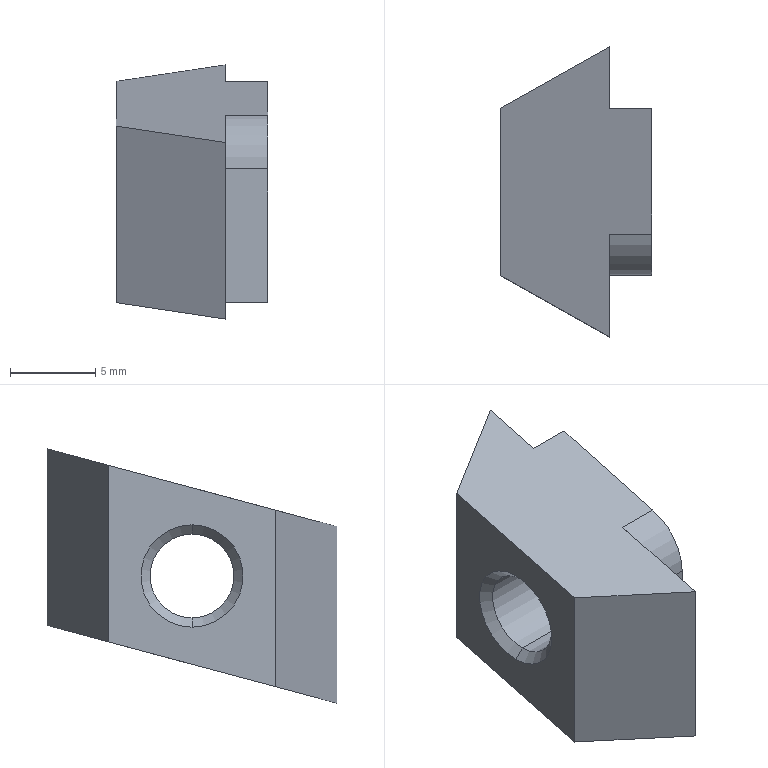Part | STEP file | 0245_019_HNTFSN8-6 | 1 solid | 18 faces | box 8.9 x 17 x 14.908 mm | volume 961.616 mm3 | plane 10 | cone 4 | cylinder 4 | commonest cylinder face diameters 4.917 x2 6.533 x2
STEP:
#1=CARTESIAN_POINT('',(0.,0.,0.));
#2=DIRECTION('',(0.,0.,1.));
#3=DIRECTION('',(1.,0.,0.));
#4=AXIS2_PLACEMENT_3D('',#1,#2,#3);
#5=CARTESIAN_POINT('',(-8.358,0.,2.459));
#6=VERTEX_POINT('',#5);
#7=CARTESIAN_POINT('',(-8.9,0.,3.));
#8=VERTEX_POINT('',#7);
#9=CARTESIAN_POINT('',(-8.9,0.,3.));
#10=DIRECTION('',(-0.7071,0.,0.7071));
#11=VECTOR('',#10,1.);
#12=LINE('',#9,#11);
#13=CARTESIAN_POINT('',(-8.9,0.,0.));
#14=DIRECTION('',(-1.,0.,0.));
#15=DIRECTION('',(0.,0.,1.));
#16=AXIS2_PLACEMENT_3D('',#13,#14,#15);
#17=CONICAL_SURFACE('',#16,3.,0.7854);
#18=CARTESIAN_POINT('',(6.283,0.));
#19=DIRECTION('',(0.,1.));
#20=VECTOR('',#19,1.);
#21=LINE('',#18,#20);
#22=(GEOMETRIC_REPRESENTATION_CONTEXT(2)PARAMETRIC_REPRESENTATION_CONTEXT()REPRESENTATION_CONTEXT('',''));
#23=DEFINITIONAL_REPRESENTATION('',(#21),#22);
#24=PCURVE('',#17,#23);
#25=CARTESIAN_POINT('',(-8.9,0.,0.));
#26=DIRECTION('',(-1.,0.,0.));
#27=DIRECTION('',(0.,0.,1.));
#28=AXIS2_PLACEMENT_3D('',#25,#26,#27);
#29=CONICAL_SURFACE('',#28,3.,0.7854);
#30=CARTESIAN_POINT('',(0.,0.));
#31=DIRECTION('',(0.,1.));
#32=VECTOR('',#31,1.);
#33=LINE('',#30,#32);
#34=(GEOMETRIC_REPRESENTATION_CONTEXT(2)PARAMETRIC_REPRESENTATION_CONTEXT()REPRESENTATION_CONTEXT('',''));
#35=DEFINITIONAL_REPRESENTATION('',(#33),#34);
#36=PCURVE('',#29,#35);
#37=SURFACE_CURVE('',#12,(#24,#36),.PCURVE_S1.);
#38=EDGE_CURVE('',#6,#8,#37,.T.);
#39=ORIENTED_EDGE('',*,*,#38,.T.);
#40=CARTESIAN_POINT('',(-8.9,0.,-3.));
#41=VERTEX_POINT('',#40);
#42=CARTESIAN_POINT('',(-8.9,0.,0.));
#43=DIRECTION('',(-1.,0.,0.));
#44=DIRECTION('',(0.,0.,1.));
#45=AXIS2_PLACEMENT_3D('',#42,#43,#44);
#46=CIRCLE('',#45,3.);
#47=CARTESIAN_POINT('',(0.,0.));
#48=DIRECTION('',(1.,0.));
#49=VECTOR('',#48,1.);
#50=LINE('',#47,#49);
#51=(GEOMETRIC_REPRESENTATION_CONTEXT(2)PARAMETRIC_REPRESENTATION_CONTEXT()REPRESENTATION_CONTEXT('',''));
#52=DEFINITIONAL_REPRESENTATION('',(#50),#51);
#53=PCURVE('',#17,#52);
#54=CARTESIAN_POINT('',(-8.9,0.,0.));
#55=DIRECTION('',(1.,0.,0.));
#56=DIRECTION('',(0.,0.,-1.));
#57=AXIS2_PLACEMENT_3D('',#54,#55,#56);
#58=PLANE('',#57);
#59=CARTESIAN_POINT('',(-3.,0.));
#60=CARTESIAN_POINT('',(-3.,5.196));
#61=CARTESIAN_POINT('',(1.5,2.598));
#62=CARTESIAN_POINT('',(6.,0.));
#63=CARTESIAN_POINT('',(1.5,-2.598));
#64=CARTESIAN_POINT('',(-3.,-5.196));
#65=CARTESIAN_POINT('',(-3.,0.));
#66=(BOUNDED_CURVE()B_SPLINE_CURVE(2,(#59,#60,#61,#62,#63,#64,#65),.UNSPECIFIED.,.T.,.F.)B_SPLINE_CURVE_WITH_KNOTS((1,2,2,2,2,1),(-2.094,0.,2.094,4.189,6.283,8.378),.UNSPECIFIED.)CURVE()GEOMETRIC_REPRESENTATION_ITEM()RATIONAL_B_SPLINE_CURVE((1.,0.5,1.,0.5,1.,0.5,1.))REPRESENTATION_ITEM(''));
#67=(GEOMETRIC_REPRESENTATION_CONTEXT(2)PARAMETRIC_REPRESENTATION_CONTEXT()REPRESENTATION_CONTEXT('',''));
#68=DEFINITIONAL_REPRESENTATION('',(#66),#67);
#69=PCURVE('',#58,#68);
#70=SURFACE_CURVE('',#46,(#53,#69),.PCURVE_S1.);
#71=EDGE_CURVE('',#41,#8,#70,.T.);
#72=ORIENTED_EDGE('',*,*,#71,.F.);
#73=CARTESIAN_POINT('',(-8.358,0.,-2.459));
#74=VERTEX_POINT('',#73);
#75=CARTESIAN_POINT('',(-8.9,0.,-3.));
#76=DIRECTION('',(-0.7071,0.,-0.7071));
#77=VECTOR('',#76,1.);
#78=LINE('',#75,#77);
#79=CARTESIAN_POINT('',(3.142,0.));
#80=DIRECTION('',(0.,1.));
#81=VECTOR('',#80,1.);
#82=LINE('',#79,#81);
#83=(GEOMETRIC_REPRESENTATION_CONTEXT(2)PARAMETRIC_REPRESENTATION_CONTEXT()REPRESENTATION_CONTEXT('',''));
#84=DEFINITIONAL_REPRESENTATION('',(#82),#83);
#85=PCURVE('',#17,#84);
#86=CARTESIAN_POINT('',(3.142,0.));
#87=DIRECTION('',(0.,1.));
#88=VECTOR('',#87,1.);
#89=LINE('',#86,#88);
#90=(GEOMETRIC_REPRESENTATION_CONTEXT(2)PARAMETRIC_REPRESENTATION_CONTEXT()REPRESENTATION_CONTEXT('',''));
#91=DEFINITIONAL_REPRESENTATION('',(#89),#90);
#92=PCURVE('',#29,#91);
#93=SURFACE_CURVE('',#78,(#85,#92),.PCURVE_S1.);
#94=EDGE_CURVE('',#74,#41,#93,.T.);
#95=ORIENTED_EDGE('',*,*,#94,.F.);
#96=CARTESIAN_POINT('',(-8.358,0.,0.));
#97=DIRECTION('',(-1.,0.,0.));
#98=DIRECTION('',(0.,1.,0.));
#99=AXIS2_PLACEMENT_3D('',#96,#97,#98);
#100=CIRCLE('',#99,2.459);
#101=CARTESIAN_POINT('',(1.571,-0.5415));
#102=DIRECTION('',(1.,0.));
#103=VECTOR('',#102,1.);
#104=LINE('',#101,#103);
#105=(GEOMETRIC_REPRESENTATION_CONTEXT(2)PARAMETRIC_REPRESENTATION_CONTEXT()REPRESENTATION_CONTEXT('',''));
#106=DEFINITIONAL_REPRESENTATION('',(#104),#105);
#107=PCURVE('',#17,#106);
#108=CARTESIAN_POINT('',(-4.45,0.,0.));
#109=DIRECTION('',(1.,0.,0.));
#110=DIRECTION('',(0.,0.,-1.));
#111=AXIS2_PLACEMENT_3D('',#108,#109,#110);
#112=CYLINDRICAL_SURFACE('',#111,2.458);
#113=CARTESIAN_POINT('',(7.854,-3.908));
#114=DIRECTION('',(-1.,0.));
#115=VECTOR('',#114,1.);
#116=LINE('',#113,#115);
#117=(GEOMETRIC_REPRESENTATION_CONTEXT(2)PARAMETRIC_REPRESENTATION_CONTEXT()REPRESENTATION_CONTEXT('',''));
#118=DEFINITIONAL_REPRESENTATION('',(#116),#117);
#119=PCURVE('',#112,#118);
#120=SURFACE_CURVE('',#100,(#107,#119),.PCURVE_S1.);
#121=EDGE_CURVE('',#74,#6,#120,.T.);
#122=ORIENTED_EDGE('',*,*,#121,.T.);
#123=EDGE_LOOP('',(#39,#72,#95,#122));
#124=FACE_BOUND('',#123,.F.);
#125=ADVANCED_FACE('',(#124),#17,.F.);
#126=CARTESIAN_POINT('',(-0.5415,0.,-2.458));
#127=VERTEX_POINT('',#126);
#128=CARTESIAN_POINT('',(0.,0.,-3.));
#129=VERTEX_POINT('',#128);
#130=CARTESIAN_POINT('',(0.,0.,-3.));
#131=DIRECTION('',(0.7071,0.,-0.7071));
#132=VECTOR('',#131,1.);
#133=LINE('',#130,#132);
#134=CARTESIAN_POINT('',(0.,0.,0.));
#135=DIRECTION('',(1.,0.,0.));
#136=DIRECTION('',(0.,0.,-1.));
#137=AXIS2_PLACEMENT_3D('',#134,#135,#136);
#138=CONICAL_SURFACE('',#137,3.,0.7854);
#139=CARTESIAN_POINT('',(6.283,0.));
#140=DIRECTION('',(0.,1.));
#141=VECTOR('',#140,1.);
#142=LINE('',#139,#141);
#143=(GEOMETRIC_REPRESENTATION_CONTEXT(2)PARAMETRIC_REPRESENTATION_CONTEXT()REPRESENTATION_CONTEXT('',''));
#144=DEFINITIONAL_REPRESENTATION('',(#142),#143);
#145=PCURVE('',#138,#144);
#146=CARTESIAN_POINT('',(0.,0.,0.));
#147=DIRECTION('',(1.,0.,0.));
#148=DIRECTION('',(0.,0.,-1.));
#149=AXIS2_PLACEMENT_3D('',#146,#147,#148);
#150=CONICAL_SURFACE('',#149,3.,0.7854);
#151=CARTESIAN_POINT('',(0.,0.));
#152=DIRECTION('',(0.,1.));
#153=VECTOR('',#152,1.);
#154=LINE('',#151,#153);
#155=(GEOMETRIC_REPRESENTATION_CONTEXT(2)PARAMETRIC_REPRESENTATION_CONTEXT()REPRESENTATION_CONTEXT('',''));
#156=DEFINITIONAL_REPRESENTATION('',(#154),#155);
#157=PCURVE('',#150,#156);
#158=SURFACE_CURVE('',#133,(#145,#157),.PCURVE_S1.);
#159=EDGE_CURVE('',#127,#129,#158,.T.);
#160=ORIENTED_EDGE('',*,*,#159,.T.);
#161=CARTESIAN_POINT('',(0.,0.,3.));
#162=VERTEX_POINT('',#161);
#163=CARTESIAN_POINT('',(0.,0.,0.));
#164=DIRECTION('',(-1.,0.,0.));
#165=DIRECTION('',(0.,0.,-1.));
#166=AXIS2_PLACEMENT_3D('',#163,#164,#165);
#167=CIRCLE('',#166,3.);
#168=CARTESIAN_POINT('',(6.283,0.));
#169=DIRECTION('',(-1.,0.));
#170=VECTOR('',#169,1.);
#171=LINE('',#168,#170);
#172=(GEOMETRIC_REPRESENTATION_CONTEXT(2)PARAMETRIC_REPRESENTATION_CONTEXT()REPRESENTATION_CONTEXT('',''));
#173=DEFINITIONAL_REPRESENTATION('',(#171),#172);
#174=PCURVE('',#138,#173);
#175=CARTESIAN_POINT('',(0.,0.,0.));
#176=DIRECTION('',(1.,0.,0.));
#177=DIRECTION('',(0.,0.,-1.));
#178=AXIS2_PLACEMENT_3D('',#175,#176,#177);
#179=PLANE('',#178);
#180=CARTESIAN_POINT('',(3.,0.));
#181=CARTESIAN_POINT('',(3.,-5.196));
#182=CARTESIAN_POINT('',(-1.5,-2.598));
#183=CARTESIAN_POINT('',(-6.,0.));
#184=CARTESIAN_POINT('',(-1.5,2.598));
#185=CARTESIAN_POINT('',(3.,5.196));
#186=CARTESIAN_POINT('',(3.,0.));
#187=(BOUNDED_CURVE()B_SPLINE_CURVE(2,(#180,#181,#182,#183,#184,#185,#186),.UNSPECIFIED.,.T.,.F.)B_SPLINE_CURVE_WITH_KNOTS((1,2,2,2,2,1),(-2.094,0.,2.094,4.189,6.283,8.378),.UNSPECIFIED.)CURVE()GEOMETRIC_REPRESENTATION_ITEM()RATIONAL_B_SPLINE_CURVE((1.,0.5,1.,0.5,1.,0.5,1.))REPRESENTATION_ITEM(''));
#188=(GEOMETRIC_REPRESENTATION_CONTEXT(2)PARAMETRIC_REPRESENTATION_CONTEXT()REPRESENTATION_CONTEXT('',''));
#189=DEFINITIONAL_REPRESENTATION('',(#187),#188);
#190=PCURVE('',#179,#189);
#191=SURFACE_CURVE('',#167,(#174,#190),.PCURVE_S1.);
#192=EDGE_CURVE('',#129,#162,#191,.T.);
#193=ORIENTED_EDGE('',*,*,#192,.T.);
#194=CARTESIAN_POINT('',(-0.5415,0.,2.458));
#195=VERTEX_POINT('',#194);
#196=CARTESIAN_POINT('',(0.,0.,3.));
#197=DIRECTION('',(0.7071,0.,0.7071));
#198=VECTOR('',#197,1.);
#199=LINE('',#196,#198);
#200=CARTESIAN_POINT('',(3.142,0.));
#201=DIRECTION('',(0.,1.));
#202=VECTOR('',#201,1.);
#203=LINE('',#200,#202);
#204=(GEOMETRIC_REPRESENTATION_CONTEXT(2)PARAMETRIC_REPRESENTATION_CONTEXT()REPRESENTATION_CONTEXT('',''));
#205=DEFINITIONAL_REPRESENTATION('',(#203),#204);
#206=PCURVE('',#138,#205);
#207=CARTESIAN_POINT('',(3.142,0.));
#208=DIRECTION('',(0.,1.));
#209=VECTOR('',#208,1.);
#210=LINE('',#207,#209);
#211=(GEOMETRIC_REPRESENTATION_CONTEXT(2)PARAMETRIC_REPRESENTATION_CONTEXT()REPRESENTATION_CONTEXT('',''));
#212=DEFINITIONAL_REPRESENTATION('',(#210),#211);
#213=PCURVE('',#150,#212);
#214=SURFACE_CURVE('',#199,(#206,#213),.PCURVE_S1.);
#215=EDGE_CURVE('',#195,#162,#214,.T.);
#216=ORIENTED_EDGE('',*,*,#215,.F.);
#217=CARTESIAN_POINT('',(-0.5415,0.,0.));
#218=DIRECTION('',(1.,0.,0.));
#219=DIRECTION('',(0.,1.,0.));
#220=AXIS2_PLACEMENT_3D('',#217,#218,#219);
#221=CIRCLE('',#220,2.458);
#222=CARTESIAN_POINT('',(1.571,-0.5415));
#223=DIRECTION('',(1.,0.));
#224=VECTOR('',#223,1.);
#225=LINE('',#222,#224);
#226=(GEOMETRIC_REPRESENTATION_CONTEXT(2)PARAMETRIC_REPRESENTATION_CONTEXT()REPRESENTATION_CONTEXT('',''));
#227=DEFINITIONAL_REPRESENTATION('',(#225),#226);
#228=PCURVE('',#138,#227);
#229=CARTESIAN_POINT('',(1.571,3.908));
#230=DIRECTION('',(1.,0.));
#231=VECTOR('',#230,1.);
#232=LINE('',#229,#231);
#233=(GEOMETRIC_REPRESENTATION_CONTEXT(2)PARAMETRIC_REPRESENTATION_CONTEXT()REPRESENTATION_CONTEXT('',''));
#234=DEFINITIONAL_REPRESENTATION('',(#232),#233);
#235=PCURVE('',#112,#234);
#236=SURFACE_CURVE('',#221,(#228,#235),.PCURVE_S1.);
#237=EDGE_CURVE('',#195,#127,#236,.T.);
#238=ORIENTED_EDGE('',*,*,#237,.T.);
#239=EDGE_LOOP('',(#160,#193,#216,#238));
#240=FACE_BOUND('',#239,.F.);
#241=ADVANCED_FACE('',(#240),#138,.F.);
#242=CARTESIAN_POINT('',(-4.45,0.,-2.458));
#243=DIRECTION('',(1.,0.,0.));
#244=VECTOR('',#243,1.);
#245=LINE('',#242,#244);
#246=CARTESIAN_POINT('',(6.283,0.));
#247=DIRECTION('',(0.,1.));
#248=VECTOR('',#247,1.);
#249=LINE('',#246,#248);
#250=(GEOMETRIC_REPRESENTATION_CONTEXT(2)PARAMETRIC_REPRESENTATION_CONTEXT()REPRESENTATION_CONTEXT('',''));
#251=DEFINITIONAL_REPRESENTATION('',(#249),#250);
#252=PCURVE('',#112,#251);
#253=CARTESIAN_POINT('',(-4.45,0.,0.));
#254=DIRECTION('',(1.,0.,0.));
#255=DIRECTION('',(0.,0.,-1.));
#256=AXIS2_PLACEMENT_3D('',#253,#254,#255);
#257=CYLINDRICAL_SURFACE('',#256,2.458);
#258=CARTESIAN_POINT('',(0.,0.));
#259=DIRECTION('',(0.,1.));
#260=VECTOR('',#259,1.);
#261=LINE('',#258,#260);
#262=(GEOMETRIC_REPRESENTATION_CONTEXT(2)PARAMETRIC_REPRESENTATION_CONTEXT()REPRESENTATION_CONTEXT('',''));
#263=DEFINITIONAL_REPRESENTATION('',(#261),#262);
#264=PCURVE('',#257,#263);
#265=SURFACE_CURVE('',#245,(#252,#264),.PCURVE_S1.);
#266=EDGE_CURVE('',#74,#127,#265,.T.);
#267=ORIENTED_EDGE('',*,*,#266,.T.);
#268=ORIENTED_EDGE('',*,*,#237,.F.);
#269=CARTESIAN_POINT('',(-4.45,0.,2.458));
#270=DIRECTION('',(1.,0.,0.));
#271=VECTOR('',#270,1.);
#272=LINE('',#269,#271);
#273=CARTESIAN_POINT('',(3.142,0.));
#274=DIRECTION('',(0.,1.));
#275=VECTOR('',#274,1.);
#276=LINE('',#273,#275);
#277=(GEOMETRIC_REPRESENTATION_CONTEXT(2)PARAMETRIC_REPRESENTATION_CONTEXT()REPRESENTATION_CONTEXT('',''));
#278=DEFINITIONAL_REPRESENTATION('',(#276),#277);
#279=PCURVE('',#112,#278);
#280=CARTESIAN_POINT('',(3.142,0.));
#281=DIRECTION('',(0.,1.));
#282=VECTOR('',#281,1.);
#283=LINE('',#280,#282);
#284=(GEOMETRIC_REPRESENTATION_CONTEXT(2)PARAMETRIC_REPRESENTATION_CONTEXT()REPRESENTATION_CONTEXT('',''));
#285=DEFINITIONAL_REPRESENTATION('',(#283),#284);
#286=PCURVE('',#257,#285);
#287=SURFACE_CURVE('',#272,(#279,#286),.PCURVE_S1.);
#288=EDGE_CURVE('',#6,#195,#287,.T.);
#289=ORIENTED_EDGE('',*,*,#288,.F.);
#290=ORIENTED_EDGE('',*,*,#121,.F.);
#291=EDGE_LOOP('',(#267,#268,#289,#290));
#292=FACE_BOUND('',#291,.F.);
#293=ADVANCED_FACE('',(#292),#112,.F.);
#294=CARTESIAN_POINT('',(-8.9,-4.9,3.863));
#295=VERTEX_POINT('',#294);
#296=CARTESIAN_POINT('',(-2.5,-8.5,2.899));
#297=VERTEX_POINT('',#296);
#298=CARTESIAN_POINT('',(-8.9,-4.9,3.863));
#299=DIRECTION('',(0.8642,-0.4861,-0.1302));
#300=VECTOR('',#299,1.);
#301=LINE('',#298,#300);
#302=CARTESIAN_POINT('',(0.,8.5,7.454));
#303=DIRECTION('',(0.,-0.2588,0.9659));
#304=DIRECTION('',(0.,-0.9659,-0.2588));
#305=AXIS2_PLACEMENT_3D('',#302,#303,#304);
#306=PLANE('',#305);
#307=CARTESIAN_POINT('',(13.873,-8.9));
#308=DIRECTION('',(0.5032,0.8642));
#309=VECTOR('',#308,1.);
#310=LINE('',#307,#309);
#311=(GEOMETRIC_REPRESENTATION_CONTEXT(2)PARAMETRIC_REPRESENTATION_CONTEXT()REPRESENTATION_CONTEXT('',''));
#312=DEFINITIONAL_REPRESENTATION('',(#310),#311);
#313=PCURVE('',#306,#312);
#314=CARTESIAN_POINT('',(-2.5,-8.5,20.));
#315=DIRECTION('',(0.4903,0.8716,0.));
#316=DIRECTION('',(-0.8716,0.4903,0.));
#317=AXIS2_PLACEMENT_3D('',#314,#315,#316);
#318=PLANE('',#317);
#319=CARTESIAN_POINT('',(7.343,-16.137));
#320=DIRECTION('',(-0.9915,-0.1302));
#321=VECTOR('',#320,1.);
#322=LINE('',#319,#321);
#323=(GEOMETRIC_REPRESENTATION_CONTEXT(2)PARAMETRIC_REPRESENTATION_CONTEXT()REPRESENTATION_CONTEXT('',''));
#324=DEFINITIONAL_REPRESENTATION('',(#322),#323);
#325=PCURVE('',#318,#324);
#326=SURFACE_CURVE('',#301,(#313,#325),.PCURVE_S1.);
#327=EDGE_CURVE('',#295,#297,#326,.T.);
#328=ORIENTED_EDGE('',*,*,#327,.T.);
#329=CARTESIAN_POINT('',(-2.5,-2.479,4.512));
#330=VERTEX_POINT('',#329);
#331=CARTESIAN_POINT('',(-2.5,8.5,7.454));
#332=DIRECTION('',(0.,0.9659,0.2588));
#333=VECTOR('',#332,1.);
#334=LINE('',#331,#333);
#335=CARTESIAN_POINT('',(0.,-2.5));
#336=DIRECTION('',(-1.,0.));
#337=VECTOR('',#336,1.);
#338=LINE('',#335,#337);
#339=(GEOMETRIC_REPRESENTATION_CONTEXT(2)PARAMETRIC_REPRESENTATION_CONTEXT()REPRESENTATION_CONTEXT('',''));
#340=DEFINITIONAL_REPRESENTATION('',(#338),#339);
#341=PCURVE('',#306,#340);
#342=CARTESIAN_POINT('',(-2.5,-4.9,20.));
#343=DIRECTION('',(-1.,0.,0.));
#344=DIRECTION('',(0.,0.,1.));
#345=AXIS2_PLACEMENT_3D('',#342,#343,#344);
#346=PLANE('',#345);
#347=CARTESIAN_POINT('',(-12.546,13.4));
#348=DIRECTION('',(0.2588,0.9659));
#349=VECTOR('',#348,1.);
#350=LINE('',#347,#349);
#351=(GEOMETRIC_REPRESENTATION_CONTEXT(2)PARAMETRIC_REPRESENTATION_CONTEXT()REPRESENTATION_CONTEXT('',''));
#352=DEFINITIONAL_REPRESENTATION('',(#350),#351);
#353=PCURVE('',#346,#352);
#354=SURFACE_CURVE('',#334,(#341,#353),.PCURVE_S1.);
#355=EDGE_CURVE('',#297,#330,#354,.T.);
#356=ORIENTED_EDGE('',*,*,#355,.T.);
#357=CARTESIAN_POINT('',(0.,-2.479,4.512));
#358=VERTEX_POINT('',#357);
#359=CARTESIAN_POINT('',(0.,-2.479,4.512));
#360=DIRECTION('',(1.,0.,0.));
#361=VECTOR('',#360,1.);
#362=LINE('',#359,#361);
#363=CARTESIAN_POINT('',(11.366,0.));
#364=DIRECTION('',(0.,1.));
#365=VECTOR('',#364,1.);
#366=LINE('',#363,#365);
#367=(GEOMETRIC_REPRESENTATION_CONTEXT(2)PARAMETRIC_REPRESENTATION_CONTEXT()REPRESENTATION_CONTEXT('',''));
#368=DEFINITIONAL_REPRESENTATION('',(#366),#367);
#369=PCURVE('',#306,#368);
#370=CARTESIAN_POINT('',(-2.5,-1.633,1.357));
#371=DIRECTION('',(-1.,0.,0.));
#372=DIRECTION('',(0.,0.,1.));
#373=AXIS2_PLACEMENT_3D('',#370,#371,#372);
#374=CYLINDRICAL_SURFACE('',#373,3.267);
#375=CARTESIAN_POINT('',(6.021,-2.5));
#376=DIRECTION('',(0.,-1.));
#377=VECTOR('',#376,1.);
#378=LINE('',#375,#377);
#379=(GEOMETRIC_REPRESENTATION_CONTEXT(2)PARAMETRIC_REPRESENTATION_CONTEXT()REPRESENTATION_CONTEXT('',''));
#380=DEFINITIONAL_REPRESENTATION('',(#378),#379);
#381=PCURVE('',#374,#380);
#382=SURFACE_CURVE('',#362,(#369,#381),.PCURVE_S1.);
#383=EDGE_CURVE('',#330,#358,#382,.T.);
#384=ORIENTED_EDGE('',*,*,#383,.T.);
#385=CARTESIAN_POINT('',(0.,4.9,6.489));
#386=VERTEX_POINT('',#385);
#387=CARTESIAN_POINT('',(0.,8.5,7.454));
#388=DIRECTION('',(0.,0.9659,0.2588));
#389=VECTOR('',#388,1.);
#390=LINE('',#387,#389);
#391=CARTESIAN_POINT('',(0.,0.));
#392=DIRECTION('',(-1.,0.));
#393=VECTOR('',#392,1.);
#394=LINE('',#391,#393);
#395=(GEOMETRIC_REPRESENTATION_CONTEXT(2)PARAMETRIC_REPRESENTATION_CONTEXT()REPRESENTATION_CONTEXT('',''));
#396=DEFINITIONAL_REPRESENTATION('',(#394),#395);
#397=PCURVE('',#306,#396);
#398=CARTESIAN_POINT('',(-7.454,8.5));
#399=DIRECTION('',(-0.2588,0.9659));
#400=VECTOR('',#399,1.);
#401=LINE('',#398,#400);
#402=(GEOMETRIC_REPRESENTATION_CONTEXT(2)PARAMETRIC_REPRESENTATION_CONTEXT()REPRESENTATION_CONTEXT('',''));
#403=DEFINITIONAL_REPRESENTATION('',(#401),#402);
#404=PCURVE('',#179,#403);
#405=SURFACE_CURVE('',#390,(#397,#404),.PCURVE_S1.);
#406=EDGE_CURVE('',#358,#386,#405,.T.);
#407=ORIENTED_EDGE('',*,*,#406,.T.);
#408=CARTESIAN_POINT('',(-2.5,4.9,6.489));
#409=VERTEX_POINT('',#408);
#410=CARTESIAN_POINT('',(0.,4.9,6.489));
#411=DIRECTION('',(-1.,0.,0.));
#412=VECTOR('',#411,1.);
#413=LINE('',#410,#412);
#414=CARTESIAN_POINT('',(3.727,0.));
#415=DIRECTION('',(0.,-1.));
#416=VECTOR('',#415,1.);
#417=LINE('',#414,#416);
#418=(GEOMETRIC_REPRESENTATION_CONTEXT(2)PARAMETRIC_REPRESENTATION_CONTEXT()REPRESENTATION_CONTEXT('',''));
#419=DEFINITIONAL_REPRESENTATION('',(#417),#418);
#420=PCURVE('',#306,#419);
#421=CARTESIAN_POINT('',(-2.5,4.9,20.));
#422=DIRECTION('',(0.,-1.,0.));
#423=DIRECTION('',(1.,0.,0.));
#424=AXIS2_PLACEMENT_3D('',#421,#422,#423);
#425=PLANE('',#424);
#426=CARTESIAN_POINT('',(2.5,-13.511));
#427=DIRECTION('',(-1.,0.));
#428=VECTOR('',#427,1.);
#429=LINE('',#426,#428);
#430=(GEOMETRIC_REPRESENTATION_CONTEXT(2)PARAMETRIC_REPRESENTATION_CONTEXT()REPRESENTATION_CONTEXT('',''));
#431=DEFINITIONAL_REPRESENTATION('',(#429),#430);
#432=PCURVE('',#425,#431);
#433=SURFACE_CURVE('',#413,(#420,#432),.PCURVE_S1.);
#434=EDGE_CURVE('',#386,#409,#433,.T.);
#435=ORIENTED_EDGE('',*,*,#434,.T.);
#436=CARTESIAN_POINT('',(-2.5,8.5,7.454));
#437=VERTEX_POINT('',#436);
#438=CARTESIAN_POINT('',(-2.5,8.5,7.454));
#439=DIRECTION('',(0.,0.9659,0.2588));
#440=VECTOR('',#439,1.);
#441=LINE('',#438,#440);
#442=CARTESIAN_POINT('',(0.,-2.5));
#443=DIRECTION('',(-1.,0.));
#444=VECTOR('',#443,1.);
#445=LINE('',#442,#444);
#446=(GEOMETRIC_REPRESENTATION_CONTEXT(2)PARAMETRIC_REPRESENTATION_CONTEXT()REPRESENTATION_CONTEXT('',''));
#447=DEFINITIONAL_REPRESENTATION('',(#445),#446);
#448=PCURVE('',#306,#447);
#449=CARTESIAN_POINT('',(-2.5,8.5,20.));
#450=DIRECTION('',(-1.,0.,0.));
#451=DIRECTION('',(0.,0.,1.));
#452=AXIS2_PLACEMENT_3D('',#449,#450,#451);
#453=PLANE('',#452);
#454=CARTESIAN_POINT('',(-12.546,0.));
#455=DIRECTION('',(0.2588,0.9659));
#456=VECTOR('',#455,1.);
#457=LINE('',#454,#456);
#458=(GEOMETRIC_REPRESENTATION_CONTEXT(2)PARAMETRIC_REPRESENTATION_CONTEXT()REPRESENTATION_CONTEXT('',''));
#459=DEFINITIONAL_REPRESENTATION('',(#457),#458);
#460=PCURVE('',#453,#459);
#461=SURFACE_CURVE('',#441,(#448,#460),.PCURVE_S1.);
#462=EDGE_CURVE('',#409,#437,#461,.T.);
#463=ORIENTED_EDGE('',*,*,#462,.T.);
#464=CARTESIAN_POINT('',(-8.9,4.9,6.489));
#465=VERTEX_POINT('',#464);
#466=CARTESIAN_POINT('',(-2.5,8.5,7.454));
#467=DIRECTION('',(-0.8642,-0.4861,-0.1302));
#468=VECTOR('',#467,1.);
#469=LINE('',#466,#468);
#470=CARTESIAN_POINT('',(0.,-2.5));
#471=DIRECTION('',(0.5032,-0.8642));
#472=VECTOR('',#471,1.);
#473=LINE('',#470,#472);
#474=(GEOMETRIC_REPRESENTATION_CONTEXT(2)PARAMETRIC_REPRESENTATION_CONTEXT()REPRESENTATION_CONTEXT('',''));
#475=DEFINITIONAL_REPRESENTATION('',(#473),#474);
#476=PCURVE('',#306,#475);
#477=CARTESIAN_POINT('',(-8.9,4.9,20.));
#478=DIRECTION('',(0.4903,-0.8716,0.));
#479=DIRECTION('',(0.8716,0.4903,0.));
#480=AXIS2_PLACEMENT_3D('',#477,#478,#479);
#481=PLANE('',#480);
#482=CARTESIAN_POINT('',(7.343,-12.546));
#483=DIRECTION('',(-0.9915,-0.1302));
#484=VECTOR('',#483,1.);
#485=LINE('',#482,#484);
#486=(GEOMETRIC_REPRESENTATION_CONTEXT(2)PARAMETRIC_REPRESENTATION_CONTEXT()REPRESENTATION_CONTEXT('',''));
#487=DEFINITIONAL_REPRESENTATION('',(#485),#486);
#488=PCURVE('',#481,#487);
#489=SURFACE_CURVE('',#469,(#476,#488),.PCURVE_S1.);
#490=EDGE_CURVE('',#437,#465,#489,.T.);
#491=ORIENTED_EDGE('',*,*,#490,.T.);
#492=CARTESIAN_POINT('',(-8.9,8.5,7.454));
#493=DIRECTION('',(0.,-0.9659,-0.2588));
#494=VECTOR('',#493,1.);
#495=LINE('',#492,#494);
#496=CARTESIAN_POINT('',(0.,-8.9));
#497=DIRECTION('',(1.,0.));
#498=VECTOR('',#497,1.);
#499=LINE('',#496,#498);
#500=(GEOMETRIC_REPRESENTATION_CONTEXT(2)PARAMETRIC_REPRESENTATION_CONTEXT()REPRESENTATION_CONTEXT('',''));
#501=DEFINITIONAL_REPRESENTATION('',(#499),#500);
#502=PCURVE('',#306,#501);
#503=CARTESIAN_POINT('',(-7.454,8.5));
#504=DIRECTION('',(0.2588,-0.9659));
#505=VECTOR('',#504,1.);
#506=LINE('',#503,#505);
#507=(GEOMETRIC_REPRESENTATION_CONTEXT(2)PARAMETRIC_REPRESENTATION_CONTEXT()REPRESENTATION_CONTEXT('',''));
#508=DEFINITIONAL_REPRESENTATION('',(#506),#507);
#509=PCURVE('',#58,#508);
#510=SURFACE_CURVE('',#495,(#502,#509),.PCURVE_S1.);
#511=EDGE_CURVE('',#465,#295,#510,.T.);
#512=ORIENTED_EDGE('',*,*,#511,.T.);
#513=EDGE_LOOP('',(#328,#356,#384,#407,#435,#463,#491,#512));
#514=FACE_BOUND('',#513,.T.);
#515=ADVANCED_FACE('',(#514),#306,.T.);
#516=CARTESIAN_POINT('',(-2.5,-8.5,-7.454));
#517=VERTEX_POINT('',#516);
#518=CARTESIAN_POINT('',(-2.5,-8.5,20.));
#519=DIRECTION('',(0.,0.,1.));
#520=VECTOR('',#519,1.);
#521=LINE('',#518,#520);
#522=CARTESIAN_POINT('',(0.,-3.6));
#523=DIRECTION('',(1.,0.));
#524=VECTOR('',#523,1.);
#525=LINE('',#522,#524);
#526=(GEOMETRIC_REPRESENTATION_CONTEXT(2)PARAMETRIC_REPRESENTATION_CONTEXT()REPRESENTATION_CONTEXT('',''));
#527=DEFINITIONAL_REPRESENTATION('',(#525),#526);
#528=PCURVE('',#346,#527);
#529=CARTESIAN_POINT('',(0.,0.));
#530=DIRECTION('',(0.,1.));
#531=VECTOR('',#530,1.);
#532=LINE('',#529,#531);
#533=(GEOMETRIC_REPRESENTATION_CONTEXT(2)PARAMETRIC_REPRESENTATION_CONTEXT()REPRESENTATION_CONTEXT('',''));
#534=DEFINITIONAL_REPRESENTATION('',(#532),#533);
#535=PCURVE('',#318,#534);
#536=SURFACE_CURVE('',#521,(#528,#535),.PCURVE_S1.);
#537=EDGE_CURVE('',#517,#297,#536,.T.);
#538=ORIENTED_EDGE('',*,*,#537,.F.);
#539=CARTESIAN_POINT('',(-2.5,-4.9,-6.489));
#540=VERTEX_POINT('',#539);
#541=CARTESIAN_POINT('',(-2.5,-4.9,-6.489));
#542=DIRECTION('',(0.,-0.9659,-0.2588));
#543=VECTOR('',#542,1.);
#544=LINE('',#541,#543);
#545=CARTESIAN_POINT('',(-26.489,0.));
#546=DIRECTION('',(-0.2588,-0.9659));
#547=VECTOR('',#546,1.);
#548=LINE('',#545,#547);
#549=(GEOMETRIC_REPRESENTATION_CONTEXT(2)PARAMETRIC_REPRESENTATION_CONTEXT()REPRESENTATION_CONTEXT('',''));
#550=DEFINITIONAL_REPRESENTATION('',(#548),#549);
#551=PCURVE('',#346,#550);
#552=CARTESIAN_POINT('',(0.,-8.5,-7.454));
#553=DIRECTION('',(0.,0.2588,-0.9659));
#554=DIRECTION('',(0.,0.9659,0.2588));
#555=AXIS2_PLACEMENT_3D('',#552,#553,#554);
#556=PLANE('',#555);
#557=CARTESIAN_POINT('',(3.727,-2.5));
#558=DIRECTION('',(-1.,0.));
#559=VECTOR('',#558,1.);
#560=LINE('',#557,#559);
#561=(GEOMETRIC_REPRESENTATION_CONTEXT(2)PARAMETRIC_REPRESENTATION_CONTEXT()REPRESENTATION_CONTEXT('',''));
#562=DEFINITIONAL_REPRESENTATION('',(#560),#561);
#563=PCURVE('',#556,#562);
#564=SURFACE_CURVE('',#544,(#551,#563),.PCURVE_S1.);
#565=EDGE_CURVE('',#540,#517,#564,.T.);
#566=ORIENTED_EDGE('',*,*,#565,.F.);
#567=CARTESIAN_POINT('',(-2.5,-4.9,1.357));
#568=VERTEX_POINT('',#567);
#569=CARTESIAN_POINT('',(-2.5,-4.9,20.));
#570=DIRECTION('',(0.,0.,-1.));
#571=VECTOR('',#570,1.);
#572=LINE('',#569,#571);
#573=CARTESIAN_POINT('',(0.,0.));
#574=DIRECTION('',(-1.,0.));
#575=VECTOR('',#574,1.);
#576=LINE('',#573,#575);
#577=(GEOMETRIC_REPRESENTATION_CONTEXT(2)PARAMETRIC_REPRESENTATION_CONTEXT()REPRESENTATION_CONTEXT('',''));
#578=DEFINITIONAL_REPRESENTATION('',(#576),#577);
#579=PCURVE('',#346,#578);
#580=CARTESIAN_POINT('',(0.,-4.9,20.));
#581=DIRECTION('',(0.,1.,0.));
#582=DIRECTION('',(-1.,0.,0.));
#583=AXIS2_PLACEMENT_3D('',#580,#581,#582);
#584=PLANE('',#583);
#585=CARTESIAN_POINT('',(2.5,0.));
#586=DIRECTION('',(0.,-1.));
#587=VECTOR('',#586,1.);
#588=LINE('',#585,#587);
#589=(GEOMETRIC_REPRESENTATION_CONTEXT(2)PARAMETRIC_REPRESENTATION_CONTEXT()REPRESENTATION_CONTEXT('',''));
#590=DEFINITIONAL_REPRESENTATION('',(#588),#589);
#591=PCURVE('',#584,#590);
#592=SURFACE_CURVE('',#572,(#579,#591),.PCURVE_S1.);
#593=EDGE_CURVE('',#568,#540,#592,.T.);
#594=ORIENTED_EDGE('',*,*,#593,.F.);
#595=CARTESIAN_POINT('',(-2.5,-1.633,1.357));
#596=DIRECTION('',(1.,0.,0.));
#597=DIRECTION('',(0.,0.,1.));
#598=AXIS2_PLACEMENT_3D('',#595,#596,#597);
#599=CIRCLE('',#598,3.267);
#600=CARTESIAN_POINT('',(-15.377,3.267));
#601=CARTESIAN_POINT('',(-15.377,-2.391));
#602=CARTESIAN_POINT('',(-20.277,0.4377));
#603=CARTESIAN_POINT('',(-25.177,3.267));
#604=CARTESIAN_POINT('',(-20.277,6.096));
#605=CARTESIAN_POINT('',(-15.377,8.925));
#606=CARTESIAN_POINT('',(-15.377,3.267));
#607=(BOUNDED_CURVE()B_SPLINE_CURVE(2,(#600,#601,#602,#603,#604,#605,#606),.UNSPECIFIED.,.T.,.F.)B_SPLINE_CURVE_WITH_KNOTS((1,2,2,2,2,1),(-2.094,0.,2.094,4.189,6.283,8.378),.UNSPECIFIED.)CURVE()GEOMETRIC_REPRESENTATION_ITEM()RATIONAL_B_SPLINE_CURVE((1.,0.5,1.,0.5,1.,0.5,1.))REPRESENTATION_ITEM(''));
#608=(GEOMETRIC_REPRESENTATION_CONTEXT(2)PARAMETRIC_REPRESENTATION_CONTEXT()REPRESENTATION_CONTEXT('',''));
#609=DEFINITIONAL_REPRESENTATION('',(#607),#608);
#610=PCURVE('',#346,#609);
#611=CARTESIAN_POINT('',(6.283,0.));
#612=DIRECTION('',(-1.,0.));
#613=VECTOR('',#612,1.);
#614=LINE('',#611,#613);
#615=(GEOMETRIC_REPRESENTATION_CONTEXT(2)PARAMETRIC_REPRESENTATION_CONTEXT()REPRESENTATION_CONTEXT('',''));
#616=DEFINITIONAL_REPRESENTATION('',(#614),#615);
#617=PCURVE('',#374,#616);
#618=SURFACE_CURVE('',#599,(#610,#617),.PCURVE_S1.);
#619=EDGE_CURVE('',#330,#568,#618,.T.);
#620=ORIENTED_EDGE('',*,*,#619,.F.);
#621=ORIENTED_EDGE('',*,*,#355,.F.);
#622=EDGE_LOOP('',(#538,#566,#594,#620,#621));
#623=FACE_BOUND('',#622,.T.);
#624=ADVANCED_FACE('',(#623),#346,.F.);
#625=ORIENTED_EDGE('',*,*,#537,.T.);
#626=ORIENTED_EDGE('',*,*,#327,.F.);
#627=CARTESIAN_POINT('',(-8.9,-4.9,-6.489));
#628=VERTEX_POINT('',#627);
#629=CARTESIAN_POINT('',(-8.9,-4.9,20.));
#630=DIRECTION('',(0.,0.,1.));
#631=VECTOR('',#630,1.);
#632=LINE('',#629,#631);
#633=CARTESIAN_POINT('',(7.343,0.));
#634=DIRECTION('',(0.,1.));
#635=VECTOR('',#634,1.);
#636=LINE('',#633,#635);
#637=(GEOMETRIC_REPRESENTATION_CONTEXT(2)PARAMETRIC_REPRESENTATION_CONTEXT()REPRESENTATION_CONTEXT('',''));
#638=DEFINITIONAL_REPRESENTATION('',(#636),#637);
#639=PCURVE('',#318,#638);
#640=CARTESIAN_POINT('',(-20.,-4.9));
#641=DIRECTION('',(-1.,0.));
#642=VECTOR('',#641,1.);
#643=LINE('',#640,#642);
#644=(GEOMETRIC_REPRESENTATION_CONTEXT(2)PARAMETRIC_REPRESENTATION_CONTEXT()REPRESENTATION_CONTEXT('',''));
#645=DEFINITIONAL_REPRESENTATION('',(#643),#644);
#646=PCURVE('',#58,#645);
#647=SURFACE_CURVE('',#632,(#639,#646),.PCURVE_S1.);
#648=EDGE_CURVE('',#628,#295,#647,.T.);
#649=ORIENTED_EDGE('',*,*,#648,.F.);
#650=CARTESIAN_POINT('',(-2.5,-8.5,-7.454));
#651=DIRECTION('',(-0.8642,0.4861,0.1302));
#652=VECTOR('',#651,1.);
#653=LINE('',#650,#652);
#654=CARTESIAN_POINT('',(0.,-27.454));
#655=DIRECTION('',(0.9915,0.1302));
#656=VECTOR('',#655,1.);
#657=LINE('',#654,#656);
#658=(GEOMETRIC_REPRESENTATION_CONTEXT(2)PARAMETRIC_REPRESENTATION_CONTEXT()REPRESENTATION_CONTEXT('',''));
#659=DEFINITIONAL_REPRESENTATION('',(#657),#658);
#660=PCURVE('',#318,#659);
#661=CARTESIAN_POINT('',(0.,-2.5));
#662=DIRECTION('',(0.5032,-0.8642));
#663=VECTOR('',#662,1.);
#664=LINE('',#661,#663);
#665=(GEOMETRIC_REPRESENTATION_CONTEXT(2)PARAMETRIC_REPRESENTATION_CONTEXT()REPRESENTATION_CONTEXT('',''));
#666=DEFINITIONAL_REPRESENTATION('',(#664),#665);
#667=PCURVE('',#556,#666);
#668=SURFACE_CURVE('',#653,(#660,#667),.PCURVE_S1.);
#669=EDGE_CURVE('',#517,#628,#668,.T.);
#670=ORIENTED_EDGE('',*,*,#669,.F.);
#671=EDGE_LOOP('',(#625,#626,#649,#670));
#672=FACE_BOUND('',#671,.T.);
#673=ADVANCED_FACE('',(#672),#318,.F.);
#674=CARTESIAN_POINT('',(-8.9,4.9,-3.863));
#675=VERTEX_POINT('',#674);
#676=CARTESIAN_POINT('',(-8.9,-4.9,-6.489));
#677=DIRECTION('',(0.,0.9659,0.2588));
#678=VECTOR('',#677,1.);
#679=LINE('',#676,#678);
#680=CARTESIAN_POINT('',(6.489,-4.9));
#681=DIRECTION('',(-0.2588,0.9659));
#682=VECTOR('',#681,1.);
#683=LINE('',#680,#682);
#684=(GEOMETRIC_REPRESENTATION_CONTEXT(2)PARAMETRIC_REPRESENTATION_CONTEXT()REPRESENTATION_CONTEXT('',''));
#685=DEFINITIONAL_REPRESENTATION('',(#683),#684);
#686=PCURVE('',#58,#685);
#687=CARTESIAN_POINT('',(3.727,-8.9));
#688=DIRECTION('',(1.,0.));
#689=VECTOR('',#688,1.);
#690=LINE('',#687,#689);
#691=(GEOMETRIC_REPRESENTATION_CONTEXT(2)PARAMETRIC_REPRESENTATION_CONTEXT()REPRESENTATION_CONTEXT('',''));
#692=DEFINITIONAL_REPRESENTATION('',(#690),#691);
#693=PCURVE('',#556,#692);
#694=SURFACE_CURVE('',#679,(#686,#693),.PCURVE_S1.);
#695=EDGE_CURVE('',#628,#675,#694,.T.);
#696=ORIENTED_EDGE('',*,*,#695,.F.);
#697=ORIENTED_EDGE('',*,*,#648,.T.);
#698=ORIENTED_EDGE('',*,*,#511,.F.);
#699=CARTESIAN_POINT('',(-8.9,4.9,0.));
#700=DIRECTION('',(0.,0.,1.));
#701=VECTOR('',#700,1.);
#702=LINE('',#699,#701);
#703=CARTESIAN_POINT('',(0.,4.9));
#704=DIRECTION('',(-1.,0.));
#705=VECTOR('',#704,1.);
#706=LINE('',#703,#705);
#707=(GEOMETRIC_REPRESENTATION_CONTEXT(2)PARAMETRIC_REPRESENTATION_CONTEXT()REPRESENTATION_CONTEXT('',''));
#708=DEFINITIONAL_REPRESENTATION('',(#706),#707);
#709=PCURVE('',#58,#708);
#710=CARTESIAN_POINT('',(0.,-20.));
#711=DIRECTION('',(0.,1.));
#712=VECTOR('',#711,1.);
#713=LINE('',#710,#712);
#714=(GEOMETRIC_REPRESENTATION_CONTEXT(2)PARAMETRIC_REPRESENTATION_CONTEXT()REPRESENTATION_CONTEXT('',''));
#715=DEFINITIONAL_REPRESENTATION('',(#713),#714);
#716=PCURVE('',#481,#715);
#717=SURFACE_CURVE('',#702,(#709,#716),.PCURVE_S1.);
#718=EDGE_CURVE('',#675,#465,#717,.T.);
#719=ORIENTED_EDGE('',*,*,#718,.F.);
#720=EDGE_LOOP('',(#696,#697,#698,#719));
#721=FACE_BOUND('',#720,.T.);
#722=CARTESIAN_POINT('',(-8.9,0.,0.));
#723=DIRECTION('',(-1.,0.,0.));
#724=DIRECTION('',(0.,0.,1.));
#725=AXIS2_PLACEMENT_3D('',#722,#723,#724);
#726=CIRCLE('',#725,3.);
#727=CARTESIAN_POINT('',(-3.,0.));
#728=CARTESIAN_POINT('',(-3.,5.196));
#729=CARTESIAN_POINT('',(1.5,2.598));
#730=CARTESIAN_POINT('',(6.,0.));
#731=CARTESIAN_POINT('',(1.5,-2.598));
#732=CARTESIAN_POINT('',(-3.,-5.196));
#733=CARTESIAN_POINT('',(-3.,0.));
#734=(BOUNDED_CURVE()B_SPLINE_CURVE(2,(#727,#728,#729,#730,#731,#732,#733),.UNSPECIFIED.,.T.,.F.)B_SPLINE_CURVE_WITH_KNOTS((1,2,2,2,2,1),(-2.094,0.,2.094,4.189,6.283,8.378),.UNSPECIFIED.)CURVE()GEOMETRIC_REPRESENTATION_ITEM()RATIONAL_B_SPLINE_CURVE((1.,0.5,1.,0.5,1.,0.5,1.))REPRESENTATION_ITEM(''));
#735=(GEOMETRIC_REPRESENTATION_CONTEXT(2)PARAMETRIC_REPRESENTATION_CONTEXT()REPRESENTATION_CONTEXT('',''));
#736=DEFINITIONAL_REPRESENTATION('',(#734),#735);
#737=PCURVE('',#58,#736);
#738=CARTESIAN_POINT('',(0.,0.));
#739=DIRECTION('',(1.,0.));
#740=VECTOR('',#739,1.);
#741=LINE('',#738,#740);
#742=(GEOMETRIC_REPRESENTATION_CONTEXT(2)PARAMETRIC_REPRESENTATION_CONTEXT()REPRESENTATION_CONTEXT('',''));
#743=DEFINITIONAL_REPRESENTATION('',(#741),#742);
#744=PCURVE('',#29,#743);
#745=SURFACE_CURVE('',#726,(#737,#744),.PCURVE_S1.);
#746=EDGE_CURVE('',#8,#41,#745,.T.);
#747=ORIENTED_EDGE('',*,*,#746,.F.);
#748=ORIENTED_EDGE('',*,*,#71,.F.);
#749=EDGE_LOOP('',(#747,#748));
#750=FACE_BOUND('',#749,.T.);
#751=ADVANCED_FACE('',(#721,#750),#58,.F.);
#752=ORIENTED_EDGE('',*,*,#718,.T.);
#753=ORIENTED_EDGE('',*,*,#490,.F.);
#754=CARTESIAN_POINT('',(-2.5,8.5,-2.899));
#755=VERTEX_POINT('',#754);
#756=CARTESIAN_POINT('',(-2.5,8.5,20.));
#757=DIRECTION('',(0.,0.,1.));
#758=VECTOR('',#757,1.);
#759=LINE('',#756,#758);
#760=CARTESIAN_POINT('',(7.343,0.));
#761=DIRECTION('',(0.,1.));
#762=VECTOR('',#761,1.);
#763=LINE('',#760,#762);
#764=(GEOMETRIC_REPRESENTATION_CONTEXT(2)PARAMETRIC_REPRESENTATION_CONTEXT()REPRESENTATION_CONTEXT('',''));
#765=DEFINITIONAL_REPRESENTATION('',(#763),#764);
#766=PCURVE('',#481,#765);
#767=CARTESIAN_POINT('',(0.,0.));
#768=DIRECTION('',(1.,0.));
#769=VECTOR('',#768,1.);
#770=LINE('',#767,#769);
#771=(GEOMETRIC_REPRESENTATION_CONTEXT(2)PARAMETRIC_REPRESENTATION_CONTEXT()REPRESENTATION_CONTEXT('',''));
#772=DEFINITIONAL_REPRESENTATION('',(#770),#771);
#773=PCURVE('',#453,#772);
#774=SURFACE_CURVE('',#759,(#766,#773),.PCURVE_S1.);
#775=EDGE_CURVE('',#755,#437,#774,.T.);
#776=ORIENTED_EDGE('',*,*,#775,.F.);
#777=CARTESIAN_POINT('',(-8.9,4.9,-3.863));
#778=DIRECTION('',(0.8642,0.4861,0.1302));
#779=VECTOR('',#778,1.);
#780=LINE('',#777,#779);
#781=CARTESIAN_POINT('',(0.,-23.863));
#782=DIRECTION('',(0.9915,0.1302));
#783=VECTOR('',#782,1.);
#784=LINE('',#781,#783);
#785=(GEOMETRIC_REPRESENTATION_CONTEXT(2)PARAMETRIC_REPRESENTATION_CONTEXT()REPRESENTATION_CONTEXT('',''));
#786=DEFINITIONAL_REPRESENTATION('',(#784),#785);
#787=PCURVE('',#481,#786);
#788=CARTESIAN_POINT('',(13.873,-8.9));
#789=DIRECTION('',(0.5032,0.8642));
#790=VECTOR('',#789,1.);
#791=LINE('',#788,#790);
#792=(GEOMETRIC_REPRESENTATION_CONTEXT(2)PARAMETRIC_REPRESENTATION_CONTEXT()REPRESENTATION_CONTEXT('',''));
#793=DEFINITIONAL_REPRESENTATION('',(#791),#792);
#794=PCURVE('',#556,#793);
#795=SURFACE_CURVE('',#780,(#787,#794),.PCURVE_S1.);
#796=EDGE_CURVE('',#675,#755,#795,.T.);
#797=ORIENTED_EDGE('',*,*,#796,.F.);
#798=EDGE_LOOP('',(#752,#753,#776,#797));
#799=FACE_BOUND('',#798,.T.);
#800=ADVANCED_FACE('',(#799),#481,.F.);
#801=CARTESIAN_POINT('',(-2.5,4.9,-1.357));
#802=VERTEX_POINT('',#801);
#803=CARTESIAN_POINT('',(-2.5,4.9,20.));
#804=DIRECTION('',(0.,0.,1.));
#805=VECTOR('',#804,1.);
#806=LINE('',#803,#805);
#807=CARTESIAN_POINT('',(0.,-3.6));
#808=DIRECTION('',(1.,0.));
#809=VECTOR('',#808,1.);
#810=LINE('',#807,#809);
#811=(GEOMETRIC_REPRESENTATION_CONTEXT(2)PARAMETRIC_REPRESENTATION_CONTEXT()REPRESENTATION_CONTEXT('',''));
#812=DEFINITIONAL_REPRESENTATION('',(#810),#811);
#813=PCURVE('',#453,#812);
#814=CARTESIAN_POINT('',(0.,0.));
#815=DIRECTION('',(0.,1.));
#816=VECTOR('',#815,1.);
#817=LINE('',#814,#816);
#818=(GEOMETRIC_REPRESENTATION_CONTEXT(2)PARAMETRIC_REPRESENTATION_CONTEXT()REPRESENTATION_CONTEXT('',''));
#819=DEFINITIONAL_REPRESENTATION('',(#817),#818);
#820=PCURVE('',#425,#819);
#821=SURFACE_CURVE('',#806,(#813,#820),.PCURVE_S1.);
#822=EDGE_CURVE('',#802,#409,#821,.T.);
#823=ORIENTED_EDGE('',*,*,#822,.F.);
#824=CARTESIAN_POINT('',(-2.5,2.479,-4.512));
#825=VERTEX_POINT('',#824);
#826=CARTESIAN_POINT('',(-2.5,1.633,-1.357));
#827=DIRECTION('',(1.,0.,0.));
#828=DIRECTION('',(0.,0.,1.));
#829=AXIS2_PLACEMENT_3D('',#826,#827,#828);
#830=CIRCLE('',#829,3.267);
#831=CARTESIAN_POINT('',(-18.09,-6.867));
#832=CARTESIAN_POINT('',(-18.09,-12.525));
#833=CARTESIAN_POINT('',(-22.99,-9.696));
#834=CARTESIAN_POINT('',(-27.89,-6.867));
#835=CARTESIAN_POINT('',(-22.99,-4.038));
#836=CARTESIAN_POINT('',(-18.09,-1.209));
#837=CARTESIAN_POINT('',(-18.09,-6.867));
#838=(BOUNDED_CURVE()B_SPLINE_CURVE(2,(#831,#832,#833,#834,#835,#836,#837),.UNSPECIFIED.,.T.,.F.)B_SPLINE_CURVE_WITH_KNOTS((1,2,2,2,2,1),(-2.094,0.,2.094,4.189,6.283,8.378),.UNSPECIFIED.)CURVE()GEOMETRIC_REPRESENTATION_ITEM()RATIONAL_B_SPLINE_CURVE((1.,0.5,1.,0.5,1.,0.5,1.))REPRESENTATION_ITEM(''));
#839=(GEOMETRIC_REPRESENTATION_CONTEXT(2)PARAMETRIC_REPRESENTATION_CONTEXT()REPRESENTATION_CONTEXT('',''));
#840=DEFINITIONAL_REPRESENTATION('',(#838),#839);
#841=PCURVE('',#453,#840);
#842=CARTESIAN_POINT('',(-2.5,1.633,-1.357));
#843=DIRECTION('',(-1.,0.,0.));
#844=DIRECTION('',(0.,0.,1.));
#845=AXIS2_PLACEMENT_3D('',#842,#843,#844);
#846=CYLINDRICAL_SURFACE('',#845,3.267);
#847=CARTESIAN_POINT('',(6.283,0.));
#848=DIRECTION('',(-1.,0.));
#849=VECTOR('',#848,1.);
#850=LINE('',#847,#849);
#851=(GEOMETRIC_REPRESENTATION_CONTEXT(2)PARAMETRIC_REPRESENTATION_CONTEXT()REPRESENTATION_CONTEXT('',''));
#852=DEFINITIONAL_REPRESENTATION('',(#850),#851);
#853=PCURVE('',#846,#852);
#854=SURFACE_CURVE('',#830,(#841,#853),.PCURVE_S1.);
#855=EDGE_CURVE('',#825,#802,#854,.T.);
#856=ORIENTED_EDGE('',*,*,#855,.F.);
#857=CARTESIAN_POINT('',(-2.5,8.5,-2.899));
#858=DIRECTION('',(0.,-0.9659,-0.2588));
#859=VECTOR('',#858,1.);
#860=LINE('',#857,#859);
#861=CARTESIAN_POINT('',(-22.899,0.));
#862=DIRECTION('',(-0.2588,-0.9659));
#863=VECTOR('',#862,1.);
#864=LINE('',#861,#863);
#865=(GEOMETRIC_REPRESENTATION_CONTEXT(2)PARAMETRIC_REPRESENTATION_CONTEXT()REPRESENTATION_CONTEXT('',''));
#866=DEFINITIONAL_REPRESENTATION('',(#864),#865);
#867=PCURVE('',#453,#866);
#868=CARTESIAN_POINT('',(17.6,-2.5));
#869=DIRECTION('',(-1.,0.));
#870=VECTOR('',#869,1.);
#871=LINE('',#868,#870);
#872=(GEOMETRIC_REPRESENTATION_CONTEXT(2)PARAMETRIC_REPRESENTATION_CONTEXT()REPRESENTATION_CONTEXT('',''));
#873=DEFINITIONAL_REPRESENTATION('',(#871),#872);
#874=PCURVE('',#556,#873);
#875=SURFACE_CURVE('',#860,(#867,#874),.PCURVE_S1.);
#876=EDGE_CURVE('',#755,#825,#875,.T.);
#877=ORIENTED_EDGE('',*,*,#876,.F.);
#878=ORIENTED_EDGE('',*,*,#775,.T.);
#879=ORIENTED_EDGE('',*,*,#462,.F.);
#880=EDGE_LOOP('',(#823,#856,#877,#878,#879));
#881=FACE_BOUND('',#880,.T.);
#882=ADVANCED_FACE('',(#881),#453,.F.);
#883=ORIENTED_EDGE('',*,*,#822,.T.);
#884=ORIENTED_EDGE('',*,*,#434,.F.);
#885=CARTESIAN_POINT('',(0.,4.9,-1.357));
#886=VERTEX_POINT('',#885);
#887=CARTESIAN_POINT('',(0.,4.9,20.));
#888=DIRECTION('',(0.,0.,1.));
#889=VECTOR('',#888,1.);
#890=LINE('',#887,#889);
#891=CARTESIAN_POINT('',(2.5,0.));
#892=DIRECTION('',(0.,1.));
#893=VECTOR('',#892,1.);
#894=LINE('',#891,#893);
#895=(GEOMETRIC_REPRESENTATION_CONTEXT(2)PARAMETRIC_REPRESENTATION_CONTEXT()REPRESENTATION_CONTEXT('',''));
#896=DEFINITIONAL_REPRESENTATION('',(#894),#895);
#897=PCURVE('',#425,#896);
#898=CARTESIAN_POINT('',(-20.,4.9));
#899=DIRECTION('',(-1.,0.));
#900=VECTOR('',#899,1.);
#901=LINE('',#898,#900);
#902=(GEOMETRIC_REPRESENTATION_CONTEXT(2)PARAMETRIC_REPRESENTATION_CONTEXT()REPRESENTATION_CONTEXT('',''));
#903=DEFINITIONAL_REPRESENTATION('',(#901),#902);
#904=PCURVE('',#179,#903);
#905=SURFACE_CURVE('',#890,(#897,#904),.PCURVE_S1.);
#906=EDGE_CURVE('',#886,#386,#905,.T.);
#907=ORIENTED_EDGE('',*,*,#906,.F.);
#908=CARTESIAN_POINT('',(-2.5,4.9,-1.357));
#909=DIRECTION('',(1.,0.,0.));
#910=VECTOR('',#909,1.);
#911=LINE('',#908,#910);
#912=CARTESIAN_POINT('',(0.,-21.357));
#913=DIRECTION('',(1.,0.));
#914=VECTOR('',#913,1.);
#915=LINE('',#912,#914);
#916=(GEOMETRIC_REPRESENTATION_CONTEXT(2)PARAMETRIC_REPRESENTATION_CONTEXT()REPRESENTATION_CONTEXT('',''));
#917=DEFINITIONAL_REPRESENTATION('',(#915),#916);
#918=PCURVE('',#425,#917);
#919=CARTESIAN_POINT('',(1.571,0.));
#920=DIRECTION('',(0.,-1.));
#921=VECTOR('',#920,1.);
#922=LINE('',#919,#921);
#923=(GEOMETRIC_REPRESENTATION_CONTEXT(2)PARAMETRIC_REPRESENTATION_CONTEXT()REPRESENTATION_CONTEXT('',''));
#924=DEFINITIONAL_REPRESENTATION('',(#922),#923);
#925=PCURVE('',#846,#924);
#926=SURFACE_CURVE('',#911,(#918,#925),.PCURVE_S1.);
#927=EDGE_CURVE('',#802,#886,#926,.T.);
#928=ORIENTED_EDGE('',*,*,#927,.F.);
#929=EDGE_LOOP('',(#883,#884,#907,#928));
#930=FACE_BOUND('',#929,.T.);
#931=ADVANCED_FACE('',(#930),#425,.F.);
#932=ORIENTED_EDGE('',*,*,#906,.T.);
#933=ORIENTED_EDGE('',*,*,#406,.F.);
#934=CARTESIAN_POINT('',(0.,-4.9,1.357));
#935=VERTEX_POINT('',#934);
#936=CARTESIAN_POINT('',(0.,-1.633,1.357));
#937=DIRECTION('',(1.,0.,0.));
#938=DIRECTION('',(0.,0.,1.));
#939=AXIS2_PLACEMENT_3D('',#936,#937,#938);
#940=CIRCLE('',#939,3.267);
#941=CARTESIAN_POINT('',(-1.357,-1.633));
#942=DIRECTION('',(-1.,0.));
#943=AXIS2_PLACEMENT_2D('',#941,#942);
#944=CIRCLE('',#943,3.267);
#945=(GEOMETRIC_REPRESENTATION_CONTEXT(2)PARAMETRIC_REPRESENTATION_CONTEXT()REPRESENTATION_CONTEXT('',''));
#946=DEFINITIONAL_REPRESENTATION('',(#944),#945);
#947=PCURVE('',#179,#946);
#948=CARTESIAN_POINT('',(6.283,-2.5));
#949=DIRECTION('',(-1.,0.));
#950=VECTOR('',#949,1.);
#951=LINE('',#948,#950);
#952=(GEOMETRIC_REPRESENTATION_CONTEXT(2)PARAMETRIC_REPRESENTATION_CONTEXT()REPRESENTATION_CONTEXT('',''));
#953=DEFINITIONAL_REPRESENTATION('',(#951),#952);
#954=PCURVE('',#374,#953);
#955=SURFACE_CURVE('',#940,(#947,#954),.PCURVE_S1.);
#956=EDGE_CURVE('',#358,#935,#955,.T.);
#957=ORIENTED_EDGE('',*,*,#956,.T.);
#958=CARTESIAN_POINT('',(0.,-4.9,-6.489));
#959=VERTEX_POINT('',#958);
#960=CARTESIAN_POINT('',(0.,-4.9,0.));
#961=DIRECTION('',(0.,0.,-1.));
#962=VECTOR('',#961,1.);
#963=LINE('',#960,#962);
#964=CARTESIAN_POINT('',(0.,-4.9));
#965=DIRECTION('',(1.,0.));
#966=VECTOR('',#965,1.);
#967=LINE('',#964,#966);
#968=(GEOMETRIC_REPRESENTATION_CONTEXT(2)PARAMETRIC_REPRESENTATION_CONTEXT()REPRESENTATION_CONTEXT('',''));
#969=DEFINITIONAL_REPRESENTATION('',(#967),#968);
#970=PCURVE('',#179,#969);
#971=CARTESIAN_POINT('',(0.,-20.));
#972=DIRECTION('',(0.,-1.));
#973=VECTOR('',#972,1.);
#974=LINE('',#971,#973);
#975=(GEOMETRIC_REPRESENTATION_CONTEXT(2)PARAMETRIC_REPRESENTATION_CONTEXT()REPRESENTATION_CONTEXT('',''));
#976=DEFINITIONAL_REPRESENTATION('',(#974),#975);
#977=PCURVE('',#584,#976);
#978=SURFACE_CURVE('',#963,(#970,#977),.PCURVE_S1.);
#979=EDGE_CURVE('',#935,#959,#978,.T.);
#980=ORIENTED_EDGE('',*,*,#979,.T.);
#981=CARTESIAN_POINT('',(0.,2.479,-4.512));
#982=VERTEX_POINT('',#981);
#983=CARTESIAN_POINT('',(0.,-4.9,-6.489));
#984=DIRECTION('',(0.,0.9659,0.2588));
#985=VECTOR('',#984,1.);
#986=LINE('',#983,#985);
#987=CARTESIAN_POINT('',(6.489,-4.9));
#988=DIRECTION('',(-0.2588,0.9659));
#989=VECTOR('',#988,1.);
#990=LINE('',#987,#989);
#991=(GEOMETRIC_REPRESENTATION_CONTEXT(2)PARAMETRIC_REPRESENTATION_CONTEXT()REPRESENTATION_CONTEXT('',''));
#992=DEFINITIONAL_REPRESENTATION('',(#990),#991);
#993=PCURVE('',#179,#992);
#994=CARTESIAN_POINT('',(3.727,0.));
#995=DIRECTION('',(1.,0.));
#996=VECTOR('',#995,1.);
#997=LINE('',#994,#996);
#998=(GEOMETRIC_REPRESENTATION_CONTEXT(2)PARAMETRIC_REPRESENTATION_CONTEXT()REPRESENTATION_CONTEXT('',''));
#999=DEFINITIONAL_REPRESENTATION('',(#997),#998);
#1000=PCURVE('',#556,#999);
#1001=SURFACE_CURVE('',#986,(#993,#1000),.PCURVE_S1.);
#1002=EDGE_CURVE('',#959,#982,#1001,.T.);
#1003=ORIENTED_EDGE('',*,*,#1002,.T.);
#1004=CARTESIAN_POINT('',(0.,1.633,-1.357));
#1005=DIRECTION('',(1.,0.,0.));
#1006=DIRECTION('',(0.,0.,1.));
#1007=AXIS2_PLACEMENT_3D('',#1004,#1005,#1006);
#1008=CIRCLE('',#1007,3.267);
#1009=CARTESIAN_POINT('',(1.357,1.633));
#1010=DIRECTION('',(-1.,0.));
#1011=AXIS2_PLACEMENT_2D('',#1009,#1010);
#1012=CIRCLE('',#1011,3.267);
#1013=(GEOMETRIC_REPRESENTATION_CONTEXT(2)PARAMETRIC_REPRESENTATION_CONTEXT()REPRESENTATION_CONTEXT('',''));
#1014=DEFINITIONAL_REPRESENTATION('',(#1012),#1013);
#1015=PCURVE('',#179,#1014);
#1016=CARTESIAN_POINT('',(6.283,-2.5));
#1017=DIRECTION('',(-1.,0.));
#1018=VECTOR('',#1017,1.);
#1019=LINE('',#1016,#1018);
#1020=(GEOMETRIC_REPRESENTATION_CONTEXT(2)PARAMETRIC_REPRESENTATION_CONTEXT()REPRESENTATION_CONTEXT('',''));
#1021=DEFINITIONAL_REPRESENTATION('',(#1019),#1020);
#1022=PCURVE('',#846,#1021);
#1023=SURFACE_CURVE('',#1008,(#1015,#1022),.PCURVE_S1.);
#1024=EDGE_CURVE('',#982,#886,#1023,.T.);
#1025=ORIENTED_EDGE('',*,*,#1024,.T.);
#1026=EDGE_LOOP('',(#932,#933,#957,#980,#1003,#1025));
#1027=FACE_BOUND('',#1026,.T.);
#1028=ORIENTED_EDGE('',*,*,#192,.T.);
#1029=CARTESIAN_POINT('',(0.,0.,0.));
#1030=DIRECTION('',(-1.,0.,0.));
#1031=DIRECTION('',(0.,0.,-1.));
#1032=AXIS2_PLACEMENT_3D('',#1029,#1030,#1031);
#1033=CIRCLE('',#1032,3.);
#1034=CARTESIAN_POINT('',(3.,0.));
#1035=CARTESIAN_POINT('',(3.,-5.196));
#1036=CARTESIAN_POINT('',(-1.5,-2.598));
#1037=CARTESIAN_POINT('',(-6.,0.));
#1038=CARTESIAN_POINT('',(-1.5,2.598));
#1039=CARTESIAN_POINT('',(3.,5.196));
#1040=CARTESIAN_POINT('',(3.,0.));
#1041=(BOUNDED_CURVE()B_SPLINE_CURVE(2,(#1034,#1035,#1036,#1037,#1038,#1039,#1040),.UNSPECIFIED.,.T.,.F.)B_SPLINE_CURVE_WITH_KNOTS((1,2,2,2,2,1),(-2.094,0.,2.094,4.189,6.283,8.378),.UNSPECIFIED.)CURVE()GEOMETRIC_REPRESENTATION_ITEM()RATIONAL_B_SPLINE_CURVE((1.,0.5,1.,0.5,1.,0.5,1.))REPRESENTATION_ITEM(''));
#1042=(GEOMETRIC_REPRESENTATION_CONTEXT(2)PARAMETRIC_REPRESENTATION_CONTEXT()REPRESENTATION_CONTEXT('',''));
#1043=DEFINITIONAL_REPRESENTATION('',(#1041),#1042);
#1044=PCURVE('',#179,#1043);
#1045=CARTESIAN_POINT('',(6.283,0.));
#1046=DIRECTION('',(-1.,0.));
#1047=VECTOR('',#1046,1.);
#1048=LINE('',#1045,#1047);
#1049=(GEOMETRIC_REPRESENTATION_CONTEXT(2)PARAMETRIC_REPRESENTATION_CONTEXT()REPRESENTATION_CONTEXT('',''));
#1050=DEFINITIONAL_REPRESENTATION('',(#1048),#1049);
#1051=PCURVE('',#150,#1050);
#1052=SURFACE_CURVE('',#1033,(#1044,#1051),.PCURVE_S1.);
#1053=EDGE_CURVE('',#162,#129,#1052,.T.);
#1054=ORIENTED_EDGE('',*,*,#1053,.T.);
#1055=EDGE_LOOP('',(#1028,#1054));
#1056=FACE_BOUND('',#1055,.T.);
#1057=ADVANCED_FACE('',(#1027,#1056),#179,.T.);
#1058=ORIENTED_EDGE('',*,*,#619,.T.);
#1059=CARTESIAN_POINT('',(-2.5,-4.9,1.357));
#1060=DIRECTION('',(1.,0.,0.));
#1061=VECTOR('',#1060,1.);
#1062=LINE('',#1059,#1061);
#1063=CARTESIAN_POINT('',(4.712,0.));
#1064=DIRECTION('',(0.,-1.));
#1065=VECTOR('',#1064,1.);
#1066=LINE('',#1063,#1065);
#1067=(GEOMETRIC_REPRESENTATION_CONTEXT(2)PARAMETRIC_REPRESENTATION_CONTEXT()REPRESENTATION_CONTEXT('',''));
#1068=DEFINITIONAL_REPRESENTATION('',(#1066),#1067);
#1069=PCURVE('',#374,#1068);
#1070=CARTESIAN_POINT('',(2.5,-18.643));
#1071=DIRECTION('',(-1.,0.));
#1072=VECTOR('',#1071,1.);
#1073=LINE('',#1070,#1072);
#1074=(GEOMETRIC_REPRESENTATION_CONTEXT(2)PARAMETRIC_REPRESENTATION_CONTEXT()REPRESENTATION_CONTEXT('',''));
#1075=DEFINITIONAL_REPRESENTATION('',(#1073),#1074);
#1076=PCURVE('',#584,#1075);
#1077=SURFACE_CURVE('',#1062,(#1069,#1076),.PCURVE_S1.);
#1078=EDGE_CURVE('',#568,#935,#1077,.T.);
#1079=ORIENTED_EDGE('',*,*,#1078,.T.);
#1080=ORIENTED_EDGE('',*,*,#956,.F.);
#1081=ORIENTED_EDGE('',*,*,#383,.F.);
#1082=EDGE_LOOP('',(#1058,#1079,#1080,#1081));
#1083=FACE_BOUND('',#1082,.T.);
#1084=ADVANCED_FACE('',(#1083),#374,.T.);
#1085=ORIENTED_EDGE('',*,*,#695,.T.);
#1086=ORIENTED_EDGE('',*,*,#796,.T.);
#1087=ORIENTED_EDGE('',*,*,#876,.T.);
#1088=CARTESIAN_POINT('',(0.,2.479,-4.512));
#1089=DIRECTION('',(1.,0.,0.));
#1090=VECTOR('',#1089,1.);
#1091=LINE('',#1088,#1090);
#1092=CARTESIAN_POINT('',(11.366,0.));
#1093=DIRECTION('',(0.,1.));
#1094=VECTOR('',#1093,1.);
#1095=LINE('',#1092,#1094);
#1096=(GEOMETRIC_REPRESENTATION_CONTEXT(2)PARAMETRIC_REPRESENTATION_CONTEXT()REPRESENTATION_CONTEXT('',''));
#1097=DEFINITIONAL_REPRESENTATION('',(#1095),#1096);
#1098=PCURVE('',#556,#1097);
#1099=CARTESIAN_POINT('',(2.88,-2.5));
#1100=DIRECTION('',(0.,-1.));
#1101=VECTOR('',#1100,1.);
#1102=LINE('',#1099,#1101);
#1103=(GEOMETRIC_REPRESENTATION_CONTEXT(2)PARAMETRIC_REPRESENTATION_CONTEXT()REPRESENTATION_CONTEXT('',''));
#1104=DEFINITIONAL_REPRESENTATION('',(#1102),#1103);
#1105=PCURVE('',#846,#1104);
#1106=SURFACE_CURVE('',#1091,(#1098,#1105),.PCURVE_S1.);
#1107=EDGE_CURVE('',#825,#982,#1106,.T.);
#1108=ORIENTED_EDGE('',*,*,#1107,.T.);
#1109=ORIENTED_EDGE('',*,*,#1002,.F.);
#1110=CARTESIAN_POINT('',(0.,-4.9,-6.489));
#1111=DIRECTION('',(-1.,0.,0.));
#1112=VECTOR('',#1111,1.);
#1113=LINE('',#1110,#1112);
#1114=CARTESIAN_POINT('',(3.727,0.));
#1115=DIRECTION('',(0.,-1.));
#1116=VECTOR('',#1115,1.);
#1117=LINE('',#1114,#1116);
#1118=(GEOMETRIC_REPRESENTATION_CONTEXT(2)PARAMETRIC_REPRESENTATION_CONTEXT()REPRESENTATION_CONTEXT('',''));
#1119=DEFINITIONAL_REPRESENTATION('',(#1117),#1118);
#1120=PCURVE('',#556,#1119);
#1121=CARTESIAN_POINT('',(0.,-26.489));
#1122=DIRECTION('',(1.,0.));
#1123=VECTOR('',#1122,1.);
#1124=LINE('',#1121,#1123);
#1125=(GEOMETRIC_REPRESENTATION_CONTEXT(2)PARAMETRIC_REPRESENTATION_CONTEXT()REPRESENTATION_CONTEXT('',''));
#1126=DEFINITIONAL_REPRESENTATION('',(#1124),#1125);
#1127=PCURVE('',#584,#1126);
#1128=SURFACE_CURVE('',#1113,(#1120,#1127),.PCURVE_S1.);
#1129=EDGE_CURVE('',#959,#540,#1128,.T.);
#1130=ORIENTED_EDGE('',*,*,#1129,.T.);
#1131=ORIENTED_EDGE('',*,*,#565,.T.);
#1132=ORIENTED_EDGE('',*,*,#669,.T.);
#1133=EDGE_LOOP('',(#1085,#1086,#1087,#1108,#1109,#1130,#1131,#1132));
#1134=FACE_BOUND('',#1133,.T.);
#1135=ADVANCED_FACE('',(#1134),#556,.T.);
#1136=ORIENTED_EDGE('',*,*,#593,.T.);
#1137=ORIENTED_EDGE('',*,*,#1129,.F.);
#1138=ORIENTED_EDGE('',*,*,#979,.F.);
#1139=ORIENTED_EDGE('',*,*,#1078,.F.);
#1140=EDGE_LOOP('',(#1136,#1137,#1138,#1139));
#1141=FACE_BOUND('',#1140,.T.);
#1142=ADVANCED_FACE('',(#1141),#584,.F.);
#1143=ORIENTED_EDGE('',*,*,#746,.F.);
#1144=ORIENTED_EDGE('',*,*,#38,.F.);
#1145=CARTESIAN_POINT('',(-8.358,0.,0.));
#1146=DIRECTION('',(-1.,0.,0.));
#1147=DIRECTION('',(0.,1.,0.));
#1148=AXIS2_PLACEMENT_3D('',#1145,#1146,#1147);
#1149=CIRCLE('',#1148,2.459);
#1150=CARTESIAN_POINT('',(-4.712,-0.5415));
#1151=DIRECTION('',(1.,0.));
#1152=VECTOR('',#1151,1.);
#1153=LINE('',#1150,#1152);
#1154=(GEOMETRIC_REPRESENTATION_CONTEXT(2)PARAMETRIC_REPRESENTATION_CONTEXT()REPRESENTATION_CONTEXT('',''));
#1155=DEFINITIONAL_REPRESENTATION('',(#1153),#1154);
#1156=PCURVE('',#29,#1155);
#1157=CARTESIAN_POINT('',(7.854,-3.908));
#1158=DIRECTION('',(-1.,0.));
#1159=VECTOR('',#1158,1.);
#1160=LINE('',#1157,#1159);
#1161=(GEOMETRIC_REPRESENTATION_CONTEXT(2)PARAMETRIC_REPRESENTATION_CONTEXT()REPRESENTATION_CONTEXT('',''));
#1162=DEFINITIONAL_REPRESENTATION('',(#1160),#1161);
#1163=PCURVE('',#257,#1162);
#1164=SURFACE_CURVE('',#1149,(#1156,#1163),.PCURVE_S1.);
#1165=EDGE_CURVE('',#6,#74,#1164,.T.);
#1166=ORIENTED_EDGE('',*,*,#1165,.T.);
#1167=ORIENTED_EDGE('',*,*,#94,.T.);
#1168=EDGE_LOOP('',(#1143,#1144,#1166,#1167));
#1169=FACE_BOUND('',#1168,.F.);
#1170=ADVANCED_FACE('',(#1169),#29,.F.);
#1171=ORIENTED_EDGE('',*,*,#855,.T.);
#1172=ORIENTED_EDGE('',*,*,#927,.T.);
#1173=ORIENTED_EDGE('',*,*,#1024,.F.);
#1174=ORIENTED_EDGE('',*,*,#1107,.F.);
#1175=EDGE_LOOP('',(#1171,#1172,#1173,#1174));
#1176=FACE_BOUND('',#1175,.T.);
#1177=ADVANCED_FACE('',(#1176),#846,.T.);
#1178=ORIENTED_EDGE('',*,*,#1053,.T.);
#1179=ORIENTED_EDGE('',*,*,#159,.F.);
#1180=CARTESIAN_POINT('',(-0.5415,0.,0.));
#1181=DIRECTION('',(1.,0.,0.));
#1182=DIRECTION('',(0.,1.,0.));
#1183=AXIS2_PLACEMENT_3D('',#1180,#1181,#1182);
#1184=CIRCLE('',#1183,2.458);
#1185=CARTESIAN_POINT('',(-4.712,-0.5415));
#1186=DIRECTION('',(1.,0.));
#1187=VECTOR('',#1186,1.);
#1188=LINE('',#1185,#1187);
#1189=(GEOMETRIC_REPRESENTATION_CONTEXT(2)PARAMETRIC_REPRESENTATION_CONTEXT()REPRESENTATION_CONTEXT('',''));
#1190=DEFINITIONAL_REPRESENTATION('',(#1188),#1189);
#1191=PCURVE('',#150,#1190);
#1192=CARTESIAN_POINT('',(-4.712,3.908));
#1193=DIRECTION('',(1.,0.));
#1194=VECTOR('',#1193,1.);
#1195=LINE('',#1192,#1194);
#1196=(GEOMETRIC_REPRESENTATION_CONTEXT(2)PARAMETRIC_REPRESENTATION_CONTEXT()REPRESENTATION_CONTEXT('',''));
#1197=DEFINITIONAL_REPRESENTATION('',(#1195),#1196);
#1198=PCURVE('',#257,#1197);
#1199=SURFACE_CURVE('',#1184,(#1191,#1198),.PCURVE_S1.);
#1200=EDGE_CURVE('',#127,#195,#1199,.T.);
#1201=ORIENTED_EDGE('',*,*,#1200,.T.);
#1202=ORIENTED_EDGE('',*,*,#215,.T.);
#1203=EDGE_LOOP('',(#1178,#1179,#1201,#1202));
#1204=FACE_BOUND('',#1203,.F.);
#1205=ADVANCED_FACE('',(#1204),#150,.F.);
#1206=ORIENTED_EDGE('',*,*,#1200,.F.);
#1207=ORIENTED_EDGE('',*,*,#266,.F.);
#1208=ORIENTED_EDGE('',*,*,#1165,.F.);
#1209=ORIENTED_EDGE('',*,*,#288,.T.);
#1210=EDGE_LOOP('',(#1206,#1207,#1208,#1209));
#1211=FACE_BOUND('',#1210,.F.);
#1212=ADVANCED_FACE('',(#1211),#257,.F.);
#1213=CLOSED_SHELL('',(#125,#241,#293,#515,#624,#673,#751,#800,#882,#931,#1057,#1084,#1135,#1142,#1170,#1177,#1205,#1212));
#1214=MANIFOLD_SOLID_BREP('',#1213);
#1215=(LENGTH_UNIT()NAMED_UNIT(*)SI_UNIT(.MILLI.,.METRE.));
#1216=UNCERTAINTY_MEASURE_WITH_UNIT(LENGTH_MEASURE(0.0000001),#1215,'','');
#1217=(NAMED_UNIT(*)PLANE_ANGLE_UNIT()SI_UNIT($,.RADIAN.));
#1218=(NAMED_UNIT(*)SI_UNIT($,.STERADIAN.)SOLID_ANGLE_UNIT());
#1219=(GEOMETRIC_REPRESENTATION_CONTEXT(3)GLOBAL_UNCERTAINTY_ASSIGNED_CONTEXT((#1216))GLOBAL_UNIT_ASSIGNED_CONTEXT((#1215,#1217,#1218))REPRESENTATION_CONTEXT('',''));
#1220=ADVANCED_BREP_SHAPE_REPRESENTATION('',(#4,#1214),#1219);